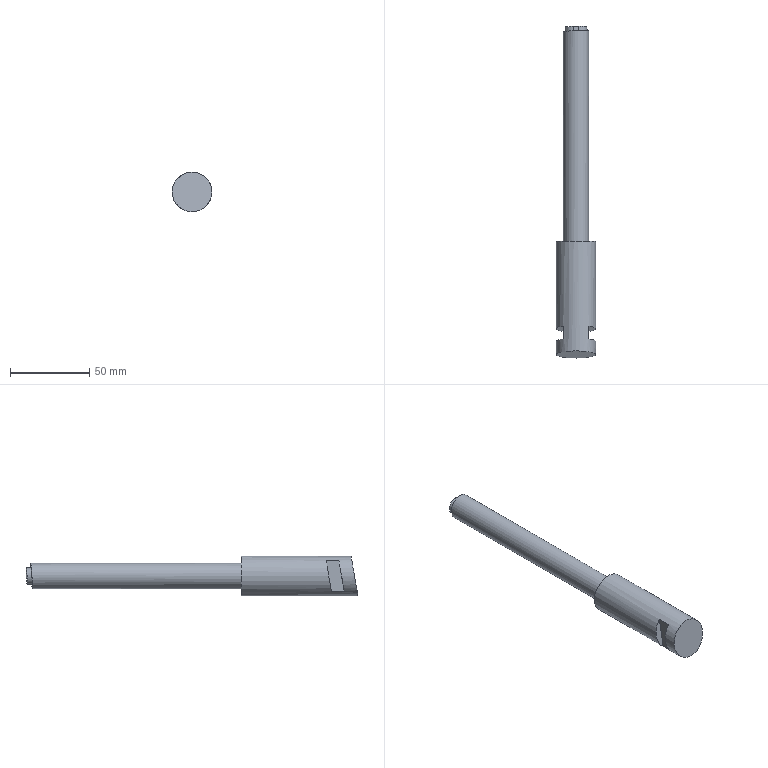Part | STEP file | solid 188 | 1 solid | 16 faces | box 25 x 209.468 x 25 mm | volume 61087 mm3 | plane 8 | spline 6 | cylinder 2 | commonest cylinder face diameters 16 x1 25 x1